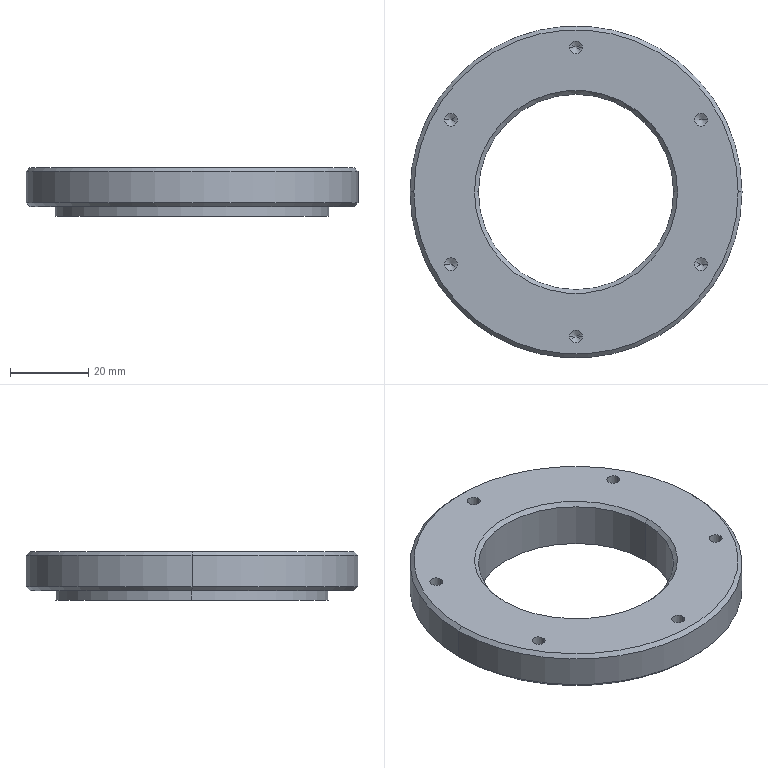Part | SolidWorks | features 3DProfileFeature 1, Chamfer 1, Extrusion 1, HoleWzd 1, ICE 1 | 1 solid | 39 faces | box 85 x 85 x 12.5 mm | volume 41153 mm3 | cylinder 18 | cone 18 | plane 3 | commonest cylinder face diameters 3.3 x12 50 x2 70 x2 85 x2
STEP:
#1=CARTESIAN_POINT('',(-35.,0.,-2.5));
#2=VERTEX_POINT('',#1);
#3=CARTESIAN_POINT('',(35.,0.,-2.5));
#4=VERTEX_POINT('',#3);
#5=CARTESIAN_POINT('',(0.,0.,-2.5));
#6=DIRECTION('',(0.,0.,-1.));
#7=DIRECTION('',(-1.,0.,0.));
#8=AXIS2_PLACEMENT_3D('',#5,#6,#7);
#9=CIRCLE('',#8,35.);
#10=EDGE_CURVE('',#2,#4,#9,.T.);
#11=ORIENTED_EDGE('',*,*,#10,.F.);
#12=CARTESIAN_POINT('',(-35.,0.,0.));
#13=VERTEX_POINT('',#12);
#14=CARTESIAN_POINT('',(-35.,0.,-2.5));
#15=DIRECTION('',(0.,0.,1.));
#16=VECTOR('',#15,1000.);
#17=LINE('',#14,#16);
#18=EDGE_CURVE('',#2,#13,#17,.T.);
#19=ORIENTED_EDGE('',*,*,#18,.T.);
#20=CARTESIAN_POINT('',(35.,0.,0.));
#21=VERTEX_POINT('',#20);
#22=CARTESIAN_POINT('',(0.,0.,0.));
#23=DIRECTION('',(0.,0.,-1.));
#24=DIRECTION('',(1.,0.,0.));
#25=AXIS2_PLACEMENT_3D('',#22,#23,#24);
#26=CIRCLE('',#25,35.);
#27=EDGE_CURVE('',#13,#21,#26,.T.);
#28=ORIENTED_EDGE('',*,*,#27,.T.);
#29=CARTESIAN_POINT('',(35.,0.,-2.5));
#30=DIRECTION('',(0.,0.,1.));
#31=VECTOR('',#30,1000.);
#32=LINE('',#29,#31);
#33=EDGE_CURVE('',#4,#21,#32,.T.);
#34=ORIENTED_EDGE('',*,*,#33,.F.);
#35=EDGE_LOOP('',(#11,#19,#28,#34));
#36=FACE_OUTER_BOUND('',#35,.T.);
#37=CARTESIAN_POINT('',(0.,0.,-2.5));
#38=DIRECTION('',(0.,0.,1.));
#39=DIRECTION('',(1.,0.,0.));
#40=AXIS2_PLACEMENT_3D('',#37,#38,#39);
#41=CYLINDRICAL_SURFACE('',#40,35.);
#42=ADVANCED_FACE('',(#36),#41,.T.);
#43=CARTESIAN_POINT('',(-1.65,37.,4.));
#44=VERTEX_POINT('',#43);
#45=CARTESIAN_POINT('',(1.65,37.,4.));
#46=VERTEX_POINT('',#45);
#47=CARTESIAN_POINT('',(0.,37.,4.));
#48=DIRECTION('',(0.,0.,1.));
#49=DIRECTION('',(1.,0.,0.));
#50=AXIS2_PLACEMENT_3D('',#47,#48,#49);
#51=CIRCLE('',#50,1.65);
#52=EDGE_CURVE('',#44,#46,#51,.T.);
#53=ORIENTED_EDGE('',*,*,#52,.F.);
#54=CARTESIAN_POINT('',(-1.65,37.,10.));
#55=VERTEX_POINT('',#54);
#56=CARTESIAN_POINT('',(-1.65,37.,10.));
#57=DIRECTION('',(0.,0.,1.));
#58=VECTOR('',#57,1000.);
#59=LINE('',#56,#58);
#60=EDGE_CURVE('',#44,#55,#59,.T.);
#61=ORIENTED_EDGE('',*,*,#60,.T.);
#62=CARTESIAN_POINT('',(1.65,37.,10.));
#63=VERTEX_POINT('',#62);
#64=CARTESIAN_POINT('',(0.,37.,10.));
#65=DIRECTION('',(0.,0.,1.));
#66=DIRECTION('',(1.,0.,0.));
#67=AXIS2_PLACEMENT_3D('',#64,#65,#66);
#68=CIRCLE('',#67,1.65);
#69=EDGE_CURVE('',#55,#63,#68,.T.);
#70=ORIENTED_EDGE('',*,*,#69,.T.);
#71=CARTESIAN_POINT('',(1.65,37.,10.));
#72=DIRECTION('',(0.,0.,1.));
#73=VECTOR('',#72,1000.);
#74=LINE('',#71,#73);
#75=EDGE_CURVE('',#46,#63,#74,.T.);
#76=ORIENTED_EDGE('',*,*,#75,.F.);
#77=EDGE_LOOP('',(#53,#61,#70,#76));
#78=FACE_OUTER_BOUND('',#77,.T.);
#79=CARTESIAN_POINT('',(0.,37.,10.));
#80=DIRECTION('',(0.,0.,1.));
#81=DIRECTION('',(1.,0.,0.));
#82=AXIS2_PLACEMENT_3D('',#79,#80,#81);
#83=CYLINDRICAL_SURFACE('',#82,1.65);
#84=ADVANCED_FACE('',(#78),#83,.F.);
#85=CARTESIAN_POINT('',(0.,37.,3.009));
#86=VERTEX_POINT('',#85);
#87=CARTESIAN_POINT('',(1.65,37.,4.));
#88=DIRECTION('',(0.8572,0.,0.515));
#89=VECTOR('',#88,1000.);
#90=LINE('',#87,#89);
#91=EDGE_CURVE('',#86,#46,#90,.T.);
#92=ORIENTED_EDGE('',*,*,#91,.F.);
#93=CARTESIAN_POINT('',(-1.65,37.,4.));
#94=DIRECTION('',(-0.8572,0.,0.515));
#95=VECTOR('',#94,1000.);
#96=LINE('',#93,#95);
#97=EDGE_CURVE('',#86,#44,#96,.T.);
#98=ORIENTED_EDGE('',*,*,#97,.T.);
#99=ORIENTED_EDGE('',*,*,#52,.T.);
#100=EDGE_LOOP('',(#92,#98,#99));
#101=FACE_OUTER_BOUND('',#100,.T.);
#102=CARTESIAN_POINT('',(0.,37.,4.));
#103=DIRECTION('',(0.,0.,1.));
#104=DIRECTION('',(1.,0.,0.));
#105=AXIS2_PLACEMENT_3D('',#102,#103,#104);
#106=CONICAL_SURFACE('',#105,1.65,1.03);
#107=ADVANCED_FACE('',(#101),#106,.F.);
#108=CARTESIAN_POINT('',(30.393,18.501,4.));
#109=VERTEX_POINT('',#108);
#110=CARTESIAN_POINT('',(33.693,18.501,4.));
#111=VERTEX_POINT('',#110);
#112=CARTESIAN_POINT('',(32.043,18.501,4.));
#113=DIRECTION('',(0.,0.,1.));
#114=DIRECTION('',(1.,0.,0.));
#115=AXIS2_PLACEMENT_3D('',#112,#113,#114);
#116=CIRCLE('',#115,1.65);
#117=EDGE_CURVE('',#109,#111,#116,.T.);
#118=ORIENTED_EDGE('',*,*,#117,.F.);
#119=CARTESIAN_POINT('',(30.393,18.501,10.));
#120=VERTEX_POINT('',#119);
#121=CARTESIAN_POINT('',(30.393,18.501,10.));
#122=DIRECTION('',(0.,0.,1.));
#123=VECTOR('',#122,1000.);
#124=LINE('',#121,#123);
#125=EDGE_CURVE('',#109,#120,#124,.T.);
#126=ORIENTED_EDGE('',*,*,#125,.T.);
#127=CARTESIAN_POINT('',(33.693,18.501,10.));
#128=VERTEX_POINT('',#127);
#129=CARTESIAN_POINT('',(32.043,18.501,10.));
#130=DIRECTION('',(0.,0.,1.));
#131=DIRECTION('',(1.,0.,0.));
#132=AXIS2_PLACEMENT_3D('',#129,#130,#131);
#133=CIRCLE('',#132,1.65);
#134=EDGE_CURVE('',#120,#128,#133,.T.);
#135=ORIENTED_EDGE('',*,*,#134,.T.);
#136=CARTESIAN_POINT('',(33.693,18.501,10.));
#137=DIRECTION('',(0.,0.,1.));
#138=VECTOR('',#137,1000.);
#139=LINE('',#136,#138);
#140=EDGE_CURVE('',#111,#128,#139,.T.);
#141=ORIENTED_EDGE('',*,*,#140,.F.);
#142=EDGE_LOOP('',(#118,#126,#135,#141));
#143=FACE_OUTER_BOUND('',#142,.T.);
#144=CARTESIAN_POINT('',(32.043,18.501,10.));
#145=DIRECTION('',(0.,0.,1.));
#146=DIRECTION('',(1.,0.,0.));
#147=AXIS2_PLACEMENT_3D('',#144,#145,#146);
#148=CYLINDRICAL_SURFACE('',#147,1.65);
#149=ADVANCED_FACE('',(#143),#148,.F.);
#150=CARTESIAN_POINT('',(32.043,18.501,3.009));
#151=VERTEX_POINT('',#150);
#152=CARTESIAN_POINT('',(33.693,18.501,4.));
#153=DIRECTION('',(0.8572,0.,0.515));
#154=VECTOR('',#153,1000.);
#155=LINE('',#152,#154);
#156=EDGE_CURVE('',#151,#111,#155,.T.);
#157=ORIENTED_EDGE('',*,*,#156,.F.);
#158=CARTESIAN_POINT('',(30.393,18.501,4.));
#159=DIRECTION('',(-0.8572,0.,0.515));
#160=VECTOR('',#159,1000.);
#161=LINE('',#158,#160);
#162=EDGE_CURVE('',#151,#109,#161,.T.);
#163=ORIENTED_EDGE('',*,*,#162,.T.);
#164=ORIENTED_EDGE('',*,*,#117,.T.);
#165=EDGE_LOOP('',(#157,#163,#164));
#166=FACE_OUTER_BOUND('',#165,.T.);
#167=CARTESIAN_POINT('',(32.043,18.501,4.));
#168=DIRECTION('',(0.,0.,1.));
#169=DIRECTION('',(1.,0.,0.));
#170=AXIS2_PLACEMENT_3D('',#167,#168,#169);
#171=CONICAL_SURFACE('',#170,1.65,1.03);
#172=ADVANCED_FACE('',(#166),#171,.F.);
#173=CARTESIAN_POINT('',(30.394,-18.499,4.));
#174=VERTEX_POINT('',#173);
#175=CARTESIAN_POINT('',(33.694,-18.499,4.));
#176=VERTEX_POINT('',#175);
#177=CARTESIAN_POINT('',(32.044,-18.499,4.));
#178=DIRECTION('',(0.,0.,1.));
#179=DIRECTION('',(1.,0.,0.));
#180=AXIS2_PLACEMENT_3D('',#177,#178,#179);
#181=CIRCLE('',#180,1.65);
#182=EDGE_CURVE('',#174,#176,#181,.T.);
#183=ORIENTED_EDGE('',*,*,#182,.F.);
#184=CARTESIAN_POINT('',(30.394,-18.499,10.));
#185=VERTEX_POINT('',#184);
#186=CARTESIAN_POINT('',(30.394,-18.499,10.));
#187=DIRECTION('',(0.,0.,1.));
#188=VECTOR('',#187,1000.);
#189=LINE('',#186,#188);
#190=EDGE_CURVE('',#174,#185,#189,.T.);
#191=ORIENTED_EDGE('',*,*,#190,.T.);
#192=CARTESIAN_POINT('',(33.694,-18.499,10.));
#193=VERTEX_POINT('',#192);
#194=CARTESIAN_POINT('',(32.044,-18.499,10.));
#195=DIRECTION('',(0.,0.,1.));
#196=DIRECTION('',(1.,0.,0.));
#197=AXIS2_PLACEMENT_3D('',#194,#195,#196);
#198=CIRCLE('',#197,1.65);
#199=EDGE_CURVE('',#185,#193,#198,.T.);
#200=ORIENTED_EDGE('',*,*,#199,.T.);
#201=CARTESIAN_POINT('',(33.694,-18.499,10.));
#202=DIRECTION('',(0.,0.,1.));
#203=VECTOR('',#202,1000.);
#204=LINE('',#201,#203);
#205=EDGE_CURVE('',#176,#193,#204,.T.);
#206=ORIENTED_EDGE('',*,*,#205,.F.);
#207=EDGE_LOOP('',(#183,#191,#200,#206));
#208=FACE_OUTER_BOUND('',#207,.T.);
#209=CARTESIAN_POINT('',(32.044,-18.499,10.));
#210=DIRECTION('',(0.,0.,1.));
#211=DIRECTION('',(1.,0.,0.));
#212=AXIS2_PLACEMENT_3D('',#209,#210,#211);
#213=CYLINDRICAL_SURFACE('',#212,1.65);
#214=ADVANCED_FACE('',(#208),#213,.F.);
#215=CARTESIAN_POINT('',(32.044,-18.499,3.009));
#216=VERTEX_POINT('',#215);
#217=CARTESIAN_POINT('',(33.694,-18.499,4.));
#218=DIRECTION('',(0.8572,0.,0.515));
#219=VECTOR('',#218,1000.);
#220=LINE('',#217,#219);
#221=EDGE_CURVE('',#216,#176,#220,.T.);
#222=ORIENTED_EDGE('',*,*,#221,.F.);
#223=CARTESIAN_POINT('',(30.394,-18.499,4.));
#224=DIRECTION('',(-0.8572,0.,0.515));
#225=VECTOR('',#224,1000.);
#226=LINE('',#223,#225);
#227=EDGE_CURVE('',#216,#174,#226,.T.);
#228=ORIENTED_EDGE('',*,*,#227,.T.);
#229=ORIENTED_EDGE('',*,*,#182,.T.);
#230=EDGE_LOOP('',(#222,#228,#229));
#231=FACE_OUTER_BOUND('',#230,.T.);
#232=CARTESIAN_POINT('',(32.044,-18.499,4.));
#233=DIRECTION('',(0.,0.,1.));
#234=DIRECTION('',(1.,0.,0.));
#235=AXIS2_PLACEMENT_3D('',#232,#233,#234);
#236=CONICAL_SURFACE('',#235,1.65,1.03);
#237=ADVANCED_FACE('',(#231),#236,.F.);
#238=CARTESIAN_POINT('',(-1.648,-37.,4.));
#239=VERTEX_POINT('',#238);
#240=CARTESIAN_POINT('',(1.652,-37.,4.));
#241=VERTEX_POINT('',#240);
#242=CARTESIAN_POINT('',(0.002,-37.,4.));
#243=DIRECTION('',(0.,0.,1.));
#244=DIRECTION('',(1.,0.,0.));
#245=AXIS2_PLACEMENT_3D('',#242,#243,#244);
#246=CIRCLE('',#245,1.65);
#247=EDGE_CURVE('',#239,#241,#246,.T.);
#248=ORIENTED_EDGE('',*,*,#247,.F.);
#249=CARTESIAN_POINT('',(-1.648,-37.,10.));
#250=VERTEX_POINT('',#249);
#251=CARTESIAN_POINT('',(-1.648,-37.,10.));
#252=DIRECTION('',(0.,0.,1.));
#253=VECTOR('',#252,1000.);
#254=LINE('',#251,#253);
#255=EDGE_CURVE('',#239,#250,#254,.T.);
#256=ORIENTED_EDGE('',*,*,#255,.T.);
#257=CARTESIAN_POINT('',(1.652,-37.,10.));
#258=VERTEX_POINT('',#257);
#259=CARTESIAN_POINT('',(0.002,-37.,10.));
#260=DIRECTION('',(0.,0.,1.));
#261=DIRECTION('',(1.,0.,0.));
#262=AXIS2_PLACEMENT_3D('',#259,#260,#261);
#263=CIRCLE('',#262,1.65);
#264=EDGE_CURVE('',#250,#258,#263,.T.);
#265=ORIENTED_EDGE('',*,*,#264,.T.);
#266=CARTESIAN_POINT('',(1.652,-37.,10.));
#267=DIRECTION('',(0.,0.,1.));
#268=VECTOR('',#267,1000.);
#269=LINE('',#266,#268);
#270=EDGE_CURVE('',#241,#258,#269,.T.);
#271=ORIENTED_EDGE('',*,*,#270,.F.);
#272=EDGE_LOOP('',(#248,#256,#265,#271));
#273=FACE_OUTER_BOUND('',#272,.T.);
#274=CARTESIAN_POINT('',(0.002,-37.,10.));
#275=DIRECTION('',(0.,0.,1.));
#276=DIRECTION('',(1.,0.,0.));
#277=AXIS2_PLACEMENT_3D('',#274,#275,#276);
#278=CYLINDRICAL_SURFACE('',#277,1.65);
#279=ADVANCED_FACE('',(#273),#278,.F.);
#280=CARTESIAN_POINT('',(0.002,-37.,3.009));
#281=VERTEX_POINT('',#280);
#282=CARTESIAN_POINT('',(1.652,-37.,4.));
#283=DIRECTION('',(0.8572,0.,0.515));
#284=VECTOR('',#283,1000.);
#285=LINE('',#282,#284);
#286=EDGE_CURVE('',#281,#241,#285,.T.);
#287=ORIENTED_EDGE('',*,*,#286,.F.);
#288=CARTESIAN_POINT('',(-1.648,-37.,4.));
#289=DIRECTION('',(-0.8572,0.,0.515));
#290=VECTOR('',#289,1000.);
#291=LINE('',#288,#290);
#292=EDGE_CURVE('',#281,#239,#291,.T.);
#293=ORIENTED_EDGE('',*,*,#292,.T.);
#294=ORIENTED_EDGE('',*,*,#247,.T.);
#295=EDGE_LOOP('',(#287,#293,#294));
#296=FACE_OUTER_BOUND('',#295,.T.);
#297=CARTESIAN_POINT('',(0.002,-37.,4.));
#298=DIRECTION('',(0.,0.,1.));
#299=DIRECTION('',(1.,0.,0.));
#300=AXIS2_PLACEMENT_3D('',#297,#298,#299);
#301=CONICAL_SURFACE('',#300,1.65,1.03);
#302=ADVANCED_FACE('',(#296),#301,.F.);
#303=CARTESIAN_POINT('',(-33.691,-18.501,4.));
#304=VERTEX_POINT('',#303);
#305=CARTESIAN_POINT('',(-30.391,-18.501,4.));
#306=VERTEX_POINT('',#305);
#307=CARTESIAN_POINT('',(-32.041,-18.501,4.));
#308=DIRECTION('',(0.,0.,1.));
#309=DIRECTION('',(1.,0.,0.));
#310=AXIS2_PLACEMENT_3D('',#307,#308,#309);
#311=CIRCLE('',#310,1.65);
#312=EDGE_CURVE('',#304,#306,#311,.T.);
#313=ORIENTED_EDGE('',*,*,#312,.F.);
#314=CARTESIAN_POINT('',(-33.691,-18.501,10.));
#315=VERTEX_POINT('',#314);
#316=CARTESIAN_POINT('',(-33.691,-18.501,10.));
#317=DIRECTION('',(0.,0.,1.));
#318=VECTOR('',#317,1000.);
#319=LINE('',#316,#318);
#320=EDGE_CURVE('',#304,#315,#319,.T.);
#321=ORIENTED_EDGE('',*,*,#320,.T.);
#322=CARTESIAN_POINT('',(-30.391,-18.501,10.));
#323=VERTEX_POINT('',#322);
#324=CARTESIAN_POINT('',(-32.041,-18.501,10.));
#325=DIRECTION('',(0.,0.,1.));
#326=DIRECTION('',(1.,0.,0.));
#327=AXIS2_PLACEMENT_3D('',#324,#325,#326);
#328=CIRCLE('',#327,1.65);
#329=EDGE_CURVE('',#315,#323,#328,.T.);
#330=ORIENTED_EDGE('',*,*,#329,.T.);
#331=CARTESIAN_POINT('',(-30.391,-18.501,10.));
#332=DIRECTION('',(0.,0.,1.));
#333=VECTOR('',#332,1000.);
#334=LINE('',#331,#333);
#335=EDGE_CURVE('',#306,#323,#334,.T.);
#336=ORIENTED_EDGE('',*,*,#335,.F.);
#337=EDGE_LOOP('',(#313,#321,#330,#336));
#338=FACE_OUTER_BOUND('',#337,.T.);
#339=CARTESIAN_POINT('',(-32.041,-18.501,10.));
#340=DIRECTION('',(0.,0.,1.));
#341=DIRECTION('',(1.,0.,0.));
#342=AXIS2_PLACEMENT_3D('',#339,#340,#341);
#343=CYLINDRICAL_SURFACE('',#342,1.65);
#344=ADVANCED_FACE('',(#338),#343,.F.);
#345=CARTESIAN_POINT('',(-32.041,-18.501,3.009));
#346=VERTEX_POINT('',#345);
#347=CARTESIAN_POINT('',(-30.391,-18.501,4.));
#348=DIRECTION('',(0.8572,0.,0.515));
#349=VECTOR('',#348,1000.);
#350=LINE('',#347,#349);
#351=EDGE_CURVE('',#346,#306,#350,.T.);
#352=ORIENTED_EDGE('',*,*,#351,.F.);
#353=CARTESIAN_POINT('',(-33.691,-18.501,4.));
#354=DIRECTION('',(-0.8572,0.,0.515));
#355=VECTOR('',#354,1000.);
#356=LINE('',#353,#355);
#357=EDGE_CURVE('',#346,#304,#356,.T.);
#358=ORIENTED_EDGE('',*,*,#357,.T.);
#359=ORIENTED_EDGE('',*,*,#312,.T.);
#360=EDGE_LOOP('',(#352,#358,#359));
#361=FACE_OUTER_BOUND('',#360,.T.);
#362=CARTESIAN_POINT('',(-32.041,-18.501,4.));
#363=DIRECTION('',(0.,0.,1.));
#364=DIRECTION('',(1.,0.,0.));
#365=AXIS2_PLACEMENT_3D('',#362,#363,#364);
#366=CONICAL_SURFACE('',#365,1.65,1.03);
#367=ADVANCED_FACE('',(#361),#366,.F.);
#368=CARTESIAN_POINT('',(-33.692,18.499,4.));
#369=VERTEX_POINT('',#368);
#370=CARTESIAN_POINT('',(-30.392,18.499,4.));
#371=VERTEX_POINT('',#370);
#372=CARTESIAN_POINT('',(-32.042,18.499,4.));
#373=DIRECTION('',(0.,0.,1.));
#374=DIRECTION('',(1.,0.,0.));
#375=AXIS2_PLACEMENT_3D('',#372,#373,#374);
#376=CIRCLE('',#375,1.65);
#377=EDGE_CURVE('',#369,#371,#376,.T.);
#378=ORIENTED_EDGE('',*,*,#377,.F.);
#379=CARTESIAN_POINT('',(-33.692,18.499,10.));
#380=VERTEX_POINT('',#379);
#381=CARTESIAN_POINT('',(-33.692,18.499,10.));
#382=DIRECTION('',(0.,0.,1.));
#383=VECTOR('',#382,1000.);
#384=LINE('',#381,#383);
#385=EDGE_CURVE('',#369,#380,#384,.T.);
#386=ORIENTED_EDGE('',*,*,#385,.T.);
#387=CARTESIAN_POINT('',(-30.392,18.499,10.));
#388=VERTEX_POINT('',#387);
#389=CARTESIAN_POINT('',(-32.042,18.499,10.));
#390=DIRECTION('',(0.,0.,1.));
#391=DIRECTION('',(1.,0.,0.));
#392=AXIS2_PLACEMENT_3D('',#389,#390,#391);
#393=CIRCLE('',#392,1.65);
#394=EDGE_CURVE('',#380,#388,#393,.T.);
#395=ORIENTED_EDGE('',*,*,#394,.T.);
#396=CARTESIAN_POINT('',(-30.392,18.499,10.));
#397=DIRECTION('',(0.,0.,1.));
#398=VECTOR('',#397,1000.);
#399=LINE('',#396,#398);
#400=EDGE_CURVE('',#371,#388,#399,.T.);
#401=ORIENTED_EDGE('',*,*,#400,.F.);
#402=EDGE_LOOP('',(#378,#386,#395,#401));
#403=FACE_OUTER_BOUND('',#402,.T.);
#404=CARTESIAN_POINT('',(-32.042,18.499,10.));
#405=DIRECTION('',(0.,0.,1.));
#406=DIRECTION('',(1.,0.,0.));
#407=AXIS2_PLACEMENT_3D('',#404,#405,#406);
#408=CYLINDRICAL_SURFACE('',#407,1.65);
#409=ADVANCED_FACE('',(#403),#408,.F.);
#410=CARTESIAN_POINT('',(-32.042,18.499,3.009));
#411=VERTEX_POINT('',#410);
#412=CARTESIAN_POINT('',(-30.392,18.499,4.));
#413=DIRECTION('',(0.8572,0.,0.515));
#414=VECTOR('',#413,1000.);
#415=LINE('',#412,#414);
#416=EDGE_CURVE('',#411,#371,#415,.T.);
#417=ORIENTED_EDGE('',*,*,#416,.F.);
#418=CARTESIAN_POINT('',(-33.692,18.499,4.));
#419=DIRECTION('',(-0.8572,0.,0.515));
#420=VECTOR('',#419,1000.);
#421=LINE('',#418,#420);
#422=EDGE_CURVE('',#411,#369,#421,.T.);
#423=ORIENTED_EDGE('',*,*,#422,.T.);
#424=ORIENTED_EDGE('',*,*,#377,.T.);
#425=EDGE_LOOP('',(#417,#423,#424));
#426=FACE_OUTER_BOUND('',#425,.T.);
#427=CARTESIAN_POINT('',(-32.042,18.499,4.));
#428=DIRECTION('',(0.,0.,1.));
#429=DIRECTION('',(1.,0.,0.));
#430=AXIS2_PLACEMENT_3D('',#427,#428,#429);
#431=CONICAL_SURFACE('',#430,1.65,1.03);
#432=ADVANCED_FACE('',(#426),#431,.F.);
#433=CARTESIAN_POINT('',(41.5,0.,10.));
#434=VERTEX_POINT('',#433);
#435=CARTESIAN_POINT('',(-41.5,0.,10.));
#436=VERTEX_POINT('',#435);
#437=CARTESIAN_POINT('',(0.,0.,10.));
#438=DIRECTION('',(0.,0.,1.));
#439=DIRECTION('',(1.,0.,0.));
#440=AXIS2_PLACEMENT_3D('',#437,#438,#439);
#441=CIRCLE('',#440,41.5);
#442=EDGE_CURVE('',#434,#436,#441,.T.);
#443=ORIENTED_EDGE('',*,*,#442,.F.);
#444=CARTESIAN_POINT('',(42.5,0.,9.));
#445=VERTEX_POINT('',#444);
#446=CARTESIAN_POINT('',(41.5,0.,10.));
#447=DIRECTION('',(0.7071,0.,-0.7071));
#448=VECTOR('',#447,1000.);
#449=LINE('',#446,#448);
#450=EDGE_CURVE('',#434,#445,#449,.T.);
#451=ORIENTED_EDGE('',*,*,#450,.T.);
#452=CARTESIAN_POINT('',(-42.5,0.,9.));
#453=VERTEX_POINT('',#452);
#454=CARTESIAN_POINT('',(0.,0.,9.));
#455=DIRECTION('',(0.,0.,-1.));
#456=DIRECTION('',(1.,0.,0.));
#457=AXIS2_PLACEMENT_3D('',#454,#455,#456);
#458=CIRCLE('',#457,42.5);
#459=EDGE_CURVE('',#453,#445,#458,.T.);
#460=ORIENTED_EDGE('',*,*,#459,.F.);
#461=CARTESIAN_POINT('',(-41.5,0.,10.));
#462=DIRECTION('',(-0.7071,0.,-0.7071));
#463=VECTOR('',#462,1000.);
#464=LINE('',#461,#463);
#465=EDGE_CURVE('',#436,#453,#464,.T.);
#466=ORIENTED_EDGE('',*,*,#465,.F.);
#467=EDGE_LOOP('',(#443,#451,#460,#466));
#468=FACE_OUTER_BOUND('',#467,.T.);
#469=CARTESIAN_POINT('',(0.,0.,10.));
#470=DIRECTION('',(0.,0.,-1.));
#471=DIRECTION('',(-1.,0.,0.));
#472=AXIS2_PLACEMENT_3D('',#469,#470,#471);
#473=CONICAL_SURFACE('',#472,41.5,0.7854);
#474=ADVANCED_FACE('',(#468),#473,.T.);
#475=CARTESIAN_POINT('',(-41.5,0.,0.));
#476=VERTEX_POINT('',#475);
#477=CARTESIAN_POINT('',(41.5,0.,0.));
#478=VERTEX_POINT('',#477);
#479=CARTESIAN_POINT('',(0.,0.,0.));
#480=DIRECTION('',(0.,0.,-1.));
#481=DIRECTION('',(1.,0.,0.));
#482=AXIS2_PLACEMENT_3D('',#479,#480,#481);
#483=CIRCLE('',#482,41.5);
#484=EDGE_CURVE('',#476,#478,#483,.T.);
#485=ORIENTED_EDGE('',*,*,#484,.F.);
#486=CARTESIAN_POINT('',(-42.5,0.,1.));
#487=VERTEX_POINT('',#486);
#488=CARTESIAN_POINT('',(-42.5,0.,1.));
#489=DIRECTION('',(-0.7071,0.,0.7071));
#490=VECTOR('',#489,1000.);
#491=LINE('',#488,#490);
#492=EDGE_CURVE('',#476,#487,#491,.T.);
#493=ORIENTED_EDGE('',*,*,#492,.T.);
#494=CARTESIAN_POINT('',(42.5,0.,1.));
#495=VERTEX_POINT('',#494);
#496=CARTESIAN_POINT('',(0.,0.,1.));
#497=DIRECTION('',(0.,0.,1.));
#498=DIRECTION('',(1.,0.,0.));
#499=AXIS2_PLACEMENT_3D('',#496,#497,#498);
#500=CIRCLE('',#499,42.5);
#501=EDGE_CURVE('',#495,#487,#500,.T.);
#502=ORIENTED_EDGE('',*,*,#501,.F.);
#503=CARTESIAN_POINT('',(42.5,0.,1.));
#504=DIRECTION('',(0.7071,0.,0.7071));
#505=VECTOR('',#504,1000.);
#506=LINE('',#503,#505);
#507=EDGE_CURVE('',#478,#495,#506,.T.);
#508=ORIENTED_EDGE('',*,*,#507,.F.);
#509=EDGE_LOOP('',(#485,#493,#502,#508));
#510=FACE_OUTER_BOUND('',#509,.T.);
#511=CARTESIAN_POINT('',(0.,0.,1.));
#512=DIRECTION('',(0.,0.,1.));
#513=DIRECTION('',(1.,0.,0.));
#514=AXIS2_PLACEMENT_3D('',#511,#512,#513);
#515=CONICAL_SURFACE('',#514,42.5,0.7854);
#516=ADVANCED_FACE('',(#510),#515,.T.);
#517=CARTESIAN_POINT('',(-25.,0.,9.));
#518=VERTEX_POINT('',#517);
#519=CARTESIAN_POINT('',(25.,0.,9.));
#520=VERTEX_POINT('',#519);
#521=CARTESIAN_POINT('',(0.,0.,9.));
#522=DIRECTION('',(0.,0.,1.));
#523=DIRECTION('',(1.,0.,0.));
#524=AXIS2_PLACEMENT_3D('',#521,#522,#523);
#525=CIRCLE('',#524,25.);
#526=EDGE_CURVE('',#518,#520,#525,.T.);
#527=ORIENTED_EDGE('',*,*,#526,.F.);
#528=CARTESIAN_POINT('',(-26.,0.,10.));
#529=VERTEX_POINT('',#528);
#530=CARTESIAN_POINT('',(-25.,0.,9.));
#531=DIRECTION('',(-0.7071,0.,0.7071));
#532=VECTOR('',#531,1000.);
#533=LINE('',#530,#532);
#534=EDGE_CURVE('',#518,#529,#533,.T.);
#535=ORIENTED_EDGE('',*,*,#534,.T.);
#536=CARTESIAN_POINT('',(26.,0.,10.));
#537=VERTEX_POINT('',#536);
#538=CARTESIAN_POINT('',(0.,0.,10.));
#539=DIRECTION('',(0.,0.,-1.));
#540=DIRECTION('',(1.,0.,0.));
#541=AXIS2_PLACEMENT_3D('',#538,#539,#540);
#542=CIRCLE('',#541,26.);
#543=EDGE_CURVE('',#537,#529,#542,.T.);
#544=ORIENTED_EDGE('',*,*,#543,.F.);
#545=CARTESIAN_POINT('',(25.,0.,9.));
#546=DIRECTION('',(0.7071,0.,0.7071));
#547=VECTOR('',#546,1000.);
#548=LINE('',#545,#547);
#549=EDGE_CURVE('',#520,#537,#548,.T.);
#550=ORIENTED_EDGE('',*,*,#549,.F.);
#551=EDGE_LOOP('',(#527,#535,#544,#550));
#552=FACE_OUTER_BOUND('',#551,.T.);
#553=CARTESIAN_POINT('',(0.,0.,9.));
#554=DIRECTION('',(0.,0.,1.));
#555=DIRECTION('',(1.,0.,0.));
#556=AXIS2_PLACEMENT_3D('',#553,#554,#555);
#557=CONICAL_SURFACE('',#556,25.,0.7854);
#558=ADVANCED_FACE('',(#552),#557,.F.);
#559=ORIENTED_EDGE('',*,*,#526,.T.);
#560=CARTESIAN_POINT('',(25.,0.,-2.5));
#561=VERTEX_POINT('',#560);
#562=CARTESIAN_POINT('',(25.,0.,10.));
#563=DIRECTION('',(0.,0.,-1.));
#564=VECTOR('',#563,1000.);
#565=LINE('',#562,#564);
#566=EDGE_CURVE('',#520,#561,#565,.T.);
#567=ORIENTED_EDGE('',*,*,#566,.T.);
#568=CARTESIAN_POINT('',(-25.,0.,-2.5));
#569=VERTEX_POINT('',#568);
#570=CARTESIAN_POINT('',(0.,0.,-2.5));
#571=DIRECTION('',(0.,0.,-1.));
#572=DIRECTION('',(-1.,0.,0.));
#573=AXIS2_PLACEMENT_3D('',#570,#571,#572);
#574=CIRCLE('',#573,25.);
#575=EDGE_CURVE('',#561,#569,#574,.T.);
#576=ORIENTED_EDGE('',*,*,#575,.T.);
#577=CARTESIAN_POINT('',(-25.,0.,10.));
#578=DIRECTION('',(0.,0.,-1.));
#579=VECTOR('',#578,1000.);
#580=LINE('',#577,#579);
#581=EDGE_CURVE('',#518,#569,#580,.T.);
#582=ORIENTED_EDGE('',*,*,#581,.F.);
#583=EDGE_LOOP('',(#559,#567,#576,#582));
#584=FACE_OUTER_BOUND('',#583,.T.);
#585=CARTESIAN_POINT('',(0.,0.,10.));
#586=DIRECTION('',(0.,0.,-1.));
#587=DIRECTION('',(-1.,0.,0.));
#588=AXIS2_PLACEMENT_3D('',#585,#586,#587);
#589=CYLINDRICAL_SURFACE('',#588,25.);
#590=ADVANCED_FACE('',(#584),#589,.F.);
#591=ORIENTED_EDGE('',*,*,#459,.T.);
#592=CARTESIAN_POINT('',(42.5,0.,10.));
#593=DIRECTION('',(0.,0.,-1.));
#594=VECTOR('',#593,1000.);
#595=LINE('',#592,#594);
#596=EDGE_CURVE('',#445,#495,#595,.T.);
#597=ORIENTED_EDGE('',*,*,#596,.T.);
#598=ORIENTED_EDGE('',*,*,#501,.T.);
#599=CARTESIAN_POINT('',(-42.5,0.,10.));
#600=DIRECTION('',(0.,0.,-1.));
#601=VECTOR('',#600,1000.);
#602=LINE('',#599,#601);
#603=EDGE_CURVE('',#453,#487,#602,.T.);
#604=ORIENTED_EDGE('',*,*,#603,.F.);
#605=EDGE_LOOP('',(#591,#597,#598,#604));
#606=FACE_OUTER_BOUND('',#605,.T.);
#607=CARTESIAN_POINT('',(0.,0.,10.));
#608=DIRECTION('',(0.,0.,-1.));
#609=DIRECTION('',(-1.,0.,0.));
#610=AXIS2_PLACEMENT_3D('',#607,#608,#609);
#611=CYLINDRICAL_SURFACE('',#610,42.5);
#612=ADVANCED_FACE('',(#606),#611,.T.);
#613=CARTESIAN_POINT('',(0.,0.,0.));
#614=DIRECTION('',(0.,0.,-1.));
#615=DIRECTION('',(1.,0.,0.));
#616=AXIS2_PLACEMENT_3D('',#613,#614,#615);
#617=CIRCLE('',#616,41.5);
#618=EDGE_CURVE('',#478,#476,#617,.T.);
#619=ORIENTED_EDGE('',*,*,#618,.T.);
#620=ORIENTED_EDGE('',*,*,#484,.T.);
#621=EDGE_LOOP('',(#619,#620));
#622=FACE_OUTER_BOUND('',#621,.T.);
#623=CARTESIAN_POINT('',(0.,0.,0.));
#624=DIRECTION('',(0.,0.,-1.));
#625=DIRECTION('',(1.,0.,0.));
#626=AXIS2_PLACEMENT_3D('',#623,#624,#625);
#627=CIRCLE('',#626,35.);
#628=EDGE_CURVE('',#21,#13,#627,.T.);
#629=ORIENTED_EDGE('',*,*,#628,.F.);
#630=ORIENTED_EDGE('',*,*,#27,.F.);
#631=EDGE_LOOP('',(#629,#630));
#632=FACE_BOUND('',#631,.T.);
#633=CARTESIAN_POINT('',(0.,0.,0.));
#634=DIRECTION('',(0.,0.,1.));
#635=DIRECTION('',(1.,0.,0.));
#636=AXIS2_PLACEMENT_3D('',#633,#634,#635);
#637=PLANE('',#636);
#638=ADVANCED_FACE('',(#622,#632),#637,.F.);
#639=CARTESIAN_POINT('',(0.,37.,10.));
#640=DIRECTION('',(0.,0.,1.));
#641=DIRECTION('',(1.,0.,0.));
#642=AXIS2_PLACEMENT_3D('',#639,#640,#641);
#643=CIRCLE('',#642,1.65);
#644=EDGE_CURVE('',#63,#55,#643,.T.);
#645=ORIENTED_EDGE('',*,*,#644,.F.);
#646=ORIENTED_EDGE('',*,*,#69,.F.);
#647=EDGE_LOOP('',(#645,#646));
#648=FACE_BOUND('',#647,.T.);
#649=CARTESIAN_POINT('',(32.043,18.501,10.));
#650=DIRECTION('',(0.,0.,1.));
#651=DIRECTION('',(1.,0.,0.));
#652=AXIS2_PLACEMENT_3D('',#649,#650,#651);
#653=CIRCLE('',#652,1.65);
#654=EDGE_CURVE('',#128,#120,#653,.T.);
#655=ORIENTED_EDGE('',*,*,#654,.F.);
#656=ORIENTED_EDGE('',*,*,#134,.F.);
#657=EDGE_LOOP('',(#655,#656));
#658=FACE_BOUND('',#657,.T.);
#659=CARTESIAN_POINT('',(32.044,-18.499,10.));
#660=DIRECTION('',(0.,0.,1.));
#661=DIRECTION('',(1.,0.,0.));
#662=AXIS2_PLACEMENT_3D('',#659,#660,#661);
#663=CIRCLE('',#662,1.65);
#664=EDGE_CURVE('',#193,#185,#663,.T.);
#665=ORIENTED_EDGE('',*,*,#664,.F.);
#666=ORIENTED_EDGE('',*,*,#199,.F.);
#667=EDGE_LOOP('',(#665,#666));
#668=FACE_BOUND('',#667,.T.);
#669=CARTESIAN_POINT('',(0.002,-37.,10.));
#670=DIRECTION('',(0.,0.,1.));
#671=DIRECTION('',(1.,0.,0.));
#672=AXIS2_PLACEMENT_3D('',#669,#670,#671);
#673=CIRCLE('',#672,1.65);
#674=EDGE_CURVE('',#258,#250,#673,.T.);
#675=ORIENTED_EDGE('',*,*,#674,.F.);
#676=ORIENTED_EDGE('',*,*,#264,.F.);
#677=EDGE_LOOP('',(#675,#676));
#678=FACE_BOUND('',#677,.T.);
#679=CARTESIAN_POINT('',(-32.041,-18.501,10.));
#680=DIRECTION('',(0.,0.,1.));
#681=DIRECTION('',(1.,0.,0.));
#682=AXIS2_PLACEMENT_3D('',#679,#680,#681);
#683=CIRCLE('',#682,1.65);
#684=EDGE_CURVE('',#323,#315,#683,.T.);
#685=ORIENTED_EDGE('',*,*,#684,.F.);
#686=ORIENTED_EDGE('',*,*,#329,.F.);
#687=EDGE_LOOP('',(#685,#686));
#688=FACE_BOUND('',#687,.T.);
#689=CARTESIAN_POINT('',(-32.042,18.499,10.));
#690=DIRECTION('',(0.,0.,1.));
#691=DIRECTION('',(1.,0.,0.));
#692=AXIS2_PLACEMENT_3D('',#689,#690,#691);
#693=CIRCLE('',#692,1.65);
#694=EDGE_CURVE('',#388,#380,#693,.T.);
#695=ORIENTED_EDGE('',*,*,#694,.F.);
#696=ORIENTED_EDGE('',*,*,#394,.F.);
#697=EDGE_LOOP('',(#695,#696));
#698=FACE_BOUND('',#697,.T.);
#699=ORIENTED_EDGE('',*,*,#543,.T.);
#700=CARTESIAN_POINT('',(0.,0.,10.));
#701=DIRECTION('',(0.,0.,-1.));
#702=DIRECTION('',(1.,0.,0.));
#703=AXIS2_PLACEMENT_3D('',#700,#701,#702);
#704=CIRCLE('',#703,26.);
#705=EDGE_CURVE('',#529,#537,#704,.T.);
#706=ORIENTED_EDGE('',*,*,#705,.T.);
#707=EDGE_LOOP('',(#699,#706));
#708=FACE_BOUND('',#707,.T.);
#709=CARTESIAN_POINT('',(0.,0.,10.));
#710=DIRECTION('',(0.,0.,1.));
#711=DIRECTION('',(1.,0.,0.));
#712=AXIS2_PLACEMENT_3D('',#709,#710,#711);
#713=CIRCLE('',#712,41.5);
#714=EDGE_CURVE('',#436,#434,#713,.T.);
#715=ORIENTED_EDGE('',*,*,#714,.T.);
#716=ORIENTED_EDGE('',*,*,#442,.T.);
#717=EDGE_LOOP('',(#715,#716));
#718=FACE_OUTER_BOUND('',#717,.T.);
#719=CARTESIAN_POINT('',(0.,0.,10.));
#720=DIRECTION('',(0.,0.,1.));
#721=DIRECTION('',(1.,0.,0.));
#722=AXIS2_PLACEMENT_3D('',#719,#720,#721);
#723=PLANE('',#722);
#724=ADVANCED_FACE('',(#648,#658,#668,#678,#688,#698,#708,#718),#723,.T.);
#725=ORIENTED_EDGE('',*,*,#596,.F.);
#726=CARTESIAN_POINT('',(0.,0.,9.));
#727=DIRECTION('',(0.,0.,-1.));
#728=DIRECTION('',(1.,0.,0.));
#729=AXIS2_PLACEMENT_3D('',#726,#727,#728);
#730=CIRCLE('',#729,42.5);
#731=EDGE_CURVE('',#445,#453,#730,.T.);
#732=ORIENTED_EDGE('',*,*,#731,.T.);
#733=ORIENTED_EDGE('',*,*,#603,.T.);
#734=CARTESIAN_POINT('',(0.,0.,1.));
#735=DIRECTION('',(0.,0.,1.));
#736=DIRECTION('',(1.,0.,0.));
#737=AXIS2_PLACEMENT_3D('',#734,#735,#736);
#738=CIRCLE('',#737,42.5);
#739=EDGE_CURVE('',#487,#495,#738,.T.);
#740=ORIENTED_EDGE('',*,*,#739,.T.);
#741=EDGE_LOOP('',(#725,#732,#733,#740));
#742=FACE_OUTER_BOUND('',#741,.T.);
#743=CARTESIAN_POINT('',(0.,0.,10.));
#744=DIRECTION('',(0.,0.,-1.));
#745=DIRECTION('',(-1.,0.,0.));
#746=AXIS2_PLACEMENT_3D('',#743,#744,#745);
#747=CYLINDRICAL_SURFACE('',#746,42.5);
#748=ADVANCED_FACE('',(#742),#747,.T.);
#749=ORIENTED_EDGE('',*,*,#566,.F.);
#750=CARTESIAN_POINT('',(0.,0.,9.));
#751=DIRECTION('',(0.,0.,1.));
#752=DIRECTION('',(1.,0.,0.));
#753=AXIS2_PLACEMENT_3D('',#750,#751,#752);
#754=CIRCLE('',#753,25.);
#755=EDGE_CURVE('',#520,#518,#754,.T.);
#756=ORIENTED_EDGE('',*,*,#755,.T.);
#757=ORIENTED_EDGE('',*,*,#581,.T.);
#758=CARTESIAN_POINT('',(0.,0.,-2.5));
#759=DIRECTION('',(0.,0.,-1.));
#760=DIRECTION('',(-1.,0.,0.));
#761=AXIS2_PLACEMENT_3D('',#758,#759,#760);
#762=CIRCLE('',#761,25.);
#763=EDGE_CURVE('',#569,#561,#762,.T.);
#764=ORIENTED_EDGE('',*,*,#763,.T.);
#765=EDGE_LOOP('',(#749,#756,#757,#764));
#766=FACE_OUTER_BOUND('',#765,.T.);
#767=CARTESIAN_POINT('',(0.,0.,10.));
#768=DIRECTION('',(0.,0.,-1.));
#769=DIRECTION('',(-1.,0.,0.));
#770=AXIS2_PLACEMENT_3D('',#767,#768,#769);
#771=CYLINDRICAL_SURFACE('',#770,25.);
#772=ADVANCED_FACE('',(#766),#771,.F.);
#773=ORIENTED_EDGE('',*,*,#534,.F.);
#774=ORIENTED_EDGE('',*,*,#755,.F.);
#775=ORIENTED_EDGE('',*,*,#549,.T.);
#776=ORIENTED_EDGE('',*,*,#705,.F.);
#777=EDGE_LOOP('',(#773,#774,#775,#776));
#778=FACE_OUTER_BOUND('',#777,.T.);
#779=CARTESIAN_POINT('',(0.,0.,9.));
#780=DIRECTION('',(0.,0.,1.));
#781=DIRECTION('',(1.,0.,0.));
#782=AXIS2_PLACEMENT_3D('',#779,#780,#781);
#783=CONICAL_SURFACE('',#782,25.,0.7854);
#784=ADVANCED_FACE('',(#778),#783,.F.);
#785=ORIENTED_EDGE('',*,*,#492,.F.);
#786=ORIENTED_EDGE('',*,*,#618,.F.);
#787=ORIENTED_EDGE('',*,*,#507,.T.);
#788=ORIENTED_EDGE('',*,*,#739,.F.);
#789=EDGE_LOOP('',(#785,#786,#787,#788));
#790=FACE_OUTER_BOUND('',#789,.T.);
#791=CARTESIAN_POINT('',(0.,0.,1.));
#792=DIRECTION('',(0.,0.,1.));
#793=DIRECTION('',(1.,0.,0.));
#794=AXIS2_PLACEMENT_3D('',#791,#792,#793);
#795=CONICAL_SURFACE('',#794,42.5,0.7854);
#796=ADVANCED_FACE('',(#790),#795,.T.);
#797=ORIENTED_EDGE('',*,*,#450,.F.);
#798=ORIENTED_EDGE('',*,*,#714,.F.);
#799=ORIENTED_EDGE('',*,*,#465,.T.);
#800=ORIENTED_EDGE('',*,*,#731,.F.);
#801=EDGE_LOOP('',(#797,#798,#799,#800));
#802=FACE_OUTER_BOUND('',#801,.T.);
#803=CARTESIAN_POINT('',(0.,0.,10.));
#804=DIRECTION('',(0.,0.,-1.));
#805=DIRECTION('',(-1.,0.,0.));
#806=AXIS2_PLACEMENT_3D('',#803,#804,#805);
#807=CONICAL_SURFACE('',#806,41.5,0.7854);
#808=ADVANCED_FACE('',(#802),#807,.T.);
#809=ORIENTED_EDGE('',*,*,#422,.F.);
#810=ORIENTED_EDGE('',*,*,#416,.T.);
#811=CARTESIAN_POINT('',(-32.042,18.499,4.));
#812=DIRECTION('',(0.,0.,1.));
#813=DIRECTION('',(1.,0.,0.));
#814=AXIS2_PLACEMENT_3D('',#811,#812,#813);
#815=CIRCLE('',#814,1.65);
#816=EDGE_CURVE('',#371,#369,#815,.T.);
#817=ORIENTED_EDGE('',*,*,#816,.T.);
#818=EDGE_LOOP('',(#809,#810,#817));
#819=FACE_OUTER_BOUND('',#818,.T.);
#820=CARTESIAN_POINT('',(-32.042,18.499,4.));
#821=DIRECTION('',(0.,0.,1.));
#822=DIRECTION('',(1.,0.,0.));
#823=AXIS2_PLACEMENT_3D('',#820,#821,#822);
#824=CONICAL_SURFACE('',#823,1.65,1.03);
#825=ADVANCED_FACE('',(#819),#824,.F.);
#826=ORIENTED_EDGE('',*,*,#385,.F.);
#827=ORIENTED_EDGE('',*,*,#816,.F.);
#828=ORIENTED_EDGE('',*,*,#400,.T.);
#829=ORIENTED_EDGE('',*,*,#694,.T.);
#830=EDGE_LOOP('',(#826,#827,#828,#829));
#831=FACE_OUTER_BOUND('',#830,.T.);
#832=CARTESIAN_POINT('',(-32.042,18.499,10.));
#833=DIRECTION('',(0.,0.,1.));
#834=DIRECTION('',(1.,0.,0.));
#835=AXIS2_PLACEMENT_3D('',#832,#833,#834);
#836=CYLINDRICAL_SURFACE('',#835,1.65);
#837=ADVANCED_FACE('',(#831),#836,.F.);
#838=ORIENTED_EDGE('',*,*,#357,.F.);
#839=ORIENTED_EDGE('',*,*,#351,.T.);
#840=CARTESIAN_POINT('',(-32.041,-18.501,4.));
#841=DIRECTION('',(0.,0.,1.));
#842=DIRECTION('',(1.,0.,0.));
#843=AXIS2_PLACEMENT_3D('',#840,#841,#842);
#844=CIRCLE('',#843,1.65);
#845=EDGE_CURVE('',#306,#304,#844,.T.);
#846=ORIENTED_EDGE('',*,*,#845,.T.);
#847=EDGE_LOOP('',(#838,#839,#846));
#848=FACE_OUTER_BOUND('',#847,.T.);
#849=CARTESIAN_POINT('',(-32.041,-18.501,4.));
#850=DIRECTION('',(0.,0.,1.));
#851=DIRECTION('',(1.,0.,0.));
#852=AXIS2_PLACEMENT_3D('',#849,#850,#851);
#853=CONICAL_SURFACE('',#852,1.65,1.03);
#854=ADVANCED_FACE('',(#848),#853,.F.);
#855=ORIENTED_EDGE('',*,*,#320,.F.);
#856=ORIENTED_EDGE('',*,*,#845,.F.);
#857=ORIENTED_EDGE('',*,*,#335,.T.);
#858=ORIENTED_EDGE('',*,*,#684,.T.);
#859=EDGE_LOOP('',(#855,#856,#857,#858));
#860=FACE_OUTER_BOUND('',#859,.T.);
#861=CARTESIAN_POINT('',(-32.041,-18.501,10.));
#862=DIRECTION('',(0.,0.,1.));
#863=DIRECTION('',(1.,0.,0.));
#864=AXIS2_PLACEMENT_3D('',#861,#862,#863);
#865=CYLINDRICAL_SURFACE('',#864,1.65);
#866=ADVANCED_FACE('',(#860),#865,.F.);
#867=ORIENTED_EDGE('',*,*,#292,.F.);
#868=ORIENTED_EDGE('',*,*,#286,.T.);
#869=CARTESIAN_POINT('',(0.002,-37.,4.));
#870=DIRECTION('',(0.,0.,1.));
#871=DIRECTION('',(1.,0.,0.));
#872=AXIS2_PLACEMENT_3D('',#869,#870,#871);
#873=CIRCLE('',#872,1.65);
#874=EDGE_CURVE('',#241,#239,#873,.T.);
#875=ORIENTED_EDGE('',*,*,#874,.T.);
#876=EDGE_LOOP('',(#867,#868,#875));
#877=FACE_OUTER_BOUND('',#876,.T.);
#878=CARTESIAN_POINT('',(0.002,-37.,4.));
#879=DIRECTION('',(0.,0.,1.));
#880=DIRECTION('',(1.,0.,0.));
#881=AXIS2_PLACEMENT_3D('',#878,#879,#880);
#882=CONICAL_SURFACE('',#881,1.65,1.03);
#883=ADVANCED_FACE('',(#877),#882,.F.);
#884=ORIENTED_EDGE('',*,*,#255,.F.);
#885=ORIENTED_EDGE('',*,*,#874,.F.);
#886=ORIENTED_EDGE('',*,*,#270,.T.);
#887=ORIENTED_EDGE('',*,*,#674,.T.);
#888=EDGE_LOOP('',(#884,#885,#886,#887));
#889=FACE_OUTER_BOUND('',#888,.T.);
#890=CARTESIAN_POINT('',(0.002,-37.,10.));
#891=DIRECTION('',(0.,0.,1.));
#892=DIRECTION('',(1.,0.,0.));
#893=AXIS2_PLACEMENT_3D('',#890,#891,#892);
#894=CYLINDRICAL_SURFACE('',#893,1.65);
#895=ADVANCED_FACE('',(#889),#894,.F.);
#896=ORIENTED_EDGE('',*,*,#227,.F.);
#897=ORIENTED_EDGE('',*,*,#221,.T.);
#898=CARTESIAN_POINT('',(32.044,-18.499,4.));
#899=DIRECTION('',(0.,0.,1.));
#900=DIRECTION('',(1.,0.,0.));
#901=AXIS2_PLACEMENT_3D('',#898,#899,#900);
#902=CIRCLE('',#901,1.65);
#903=EDGE_CURVE('',#176,#174,#902,.T.);
#904=ORIENTED_EDGE('',*,*,#903,.T.);
#905=EDGE_LOOP('',(#896,#897,#904));
#906=FACE_OUTER_BOUND('',#905,.T.);
#907=CARTESIAN_POINT('',(32.044,-18.499,4.));
#908=DIRECTION('',(0.,0.,1.));
#909=DIRECTION('',(1.,0.,0.));
#910=AXIS2_PLACEMENT_3D('',#907,#908,#909);
#911=CONICAL_SURFACE('',#910,1.65,1.03);
#912=ADVANCED_FACE('',(#906),#911,.F.);
#913=ORIENTED_EDGE('',*,*,#190,.F.);
#914=ORIENTED_EDGE('',*,*,#903,.F.);
#915=ORIENTED_EDGE('',*,*,#205,.T.);
#916=ORIENTED_EDGE('',*,*,#664,.T.);
#917=EDGE_LOOP('',(#913,#914,#915,#916));
#918=FACE_OUTER_BOUND('',#917,.T.);
#919=CARTESIAN_POINT('',(32.044,-18.499,10.));
#920=DIRECTION('',(0.,0.,1.));
#921=DIRECTION('',(1.,0.,0.));
#922=AXIS2_PLACEMENT_3D('',#919,#920,#921);
#923=CYLINDRICAL_SURFACE('',#922,1.65);
#924=ADVANCED_FACE('',(#918),#923,.F.);
#925=ORIENTED_EDGE('',*,*,#162,.F.);
#926=ORIENTED_EDGE('',*,*,#156,.T.);
#927=CARTESIAN_POINT('',(32.043,18.501,4.));
#928=DIRECTION('',(0.,0.,1.));
#929=DIRECTION('',(1.,0.,0.));
#930=AXIS2_PLACEMENT_3D('',#927,#928,#929);
#931=CIRCLE('',#930,1.65);
#932=EDGE_CURVE('',#111,#109,#931,.T.);
#933=ORIENTED_EDGE('',*,*,#932,.T.);
#934=EDGE_LOOP('',(#925,#926,#933));
#935=FACE_OUTER_BOUND('',#934,.T.);
#936=CARTESIAN_POINT('',(32.043,18.501,4.));
#937=DIRECTION('',(0.,0.,1.));
#938=DIRECTION('',(1.,0.,0.));
#939=AXIS2_PLACEMENT_3D('',#936,#937,#938);
#940=CONICAL_SURFACE('',#939,1.65,1.03);
#941=ADVANCED_FACE('',(#935),#940,.F.);
#942=ORIENTED_EDGE('',*,*,#125,.F.);
#943=ORIENTED_EDGE('',*,*,#932,.F.);
#944=ORIENTED_EDGE('',*,*,#140,.T.);
#945=ORIENTED_EDGE('',*,*,#654,.T.);
#946=EDGE_LOOP('',(#942,#943,#944,#945));
#947=FACE_OUTER_BOUND('',#946,.T.);
#948=CARTESIAN_POINT('',(32.043,18.501,10.));
#949=DIRECTION('',(0.,0.,1.));
#950=DIRECTION('',(1.,0.,0.));
#951=AXIS2_PLACEMENT_3D('',#948,#949,#950);
#952=CYLINDRICAL_SURFACE('',#951,1.65);
#953=ADVANCED_FACE('',(#947),#952,.F.);
#954=ORIENTED_EDGE('',*,*,#97,.F.);
#955=ORIENTED_EDGE('',*,*,#91,.T.);
#956=CARTESIAN_POINT('',(0.,37.,4.));
#957=DIRECTION('',(0.,0.,1.));
#958=DIRECTION('',(1.,0.,0.));
#959=AXIS2_PLACEMENT_3D('',#956,#957,#958);
#960=CIRCLE('',#959,1.65);
#961=EDGE_CURVE('',#46,#44,#960,.T.);
#962=ORIENTED_EDGE('',*,*,#961,.T.);
#963=EDGE_LOOP('',(#954,#955,#962));
#964=FACE_OUTER_BOUND('',#963,.T.);
#965=CARTESIAN_POINT('',(0.,37.,4.));
#966=DIRECTION('',(0.,0.,1.));
#967=DIRECTION('',(1.,0.,0.));
#968=AXIS2_PLACEMENT_3D('',#965,#966,#967);
#969=CONICAL_SURFACE('',#968,1.65,1.03);
#970=ADVANCED_FACE('',(#964),#969,.F.);
#971=ORIENTED_EDGE('',*,*,#60,.F.);
#972=ORIENTED_EDGE('',*,*,#961,.F.);
#973=ORIENTED_EDGE('',*,*,#75,.T.);
#974=ORIENTED_EDGE('',*,*,#644,.T.);
#975=EDGE_LOOP('',(#971,#972,#973,#974));
#976=FACE_OUTER_BOUND('',#975,.T.);
#977=CARTESIAN_POINT('',(0.,37.,10.));
#978=DIRECTION('',(0.,0.,1.));
#979=DIRECTION('',(1.,0.,0.));
#980=AXIS2_PLACEMENT_3D('',#977,#978,#979);
#981=CYLINDRICAL_SURFACE('',#980,1.65);
#982=ADVANCED_FACE('',(#976),#981,.F.);
#983=CARTESIAN_POINT('',(0.,0.,-2.5));
#984=DIRECTION('',(0.,0.,-1.));
#985=DIRECTION('',(-1.,0.,0.));
#986=AXIS2_PLACEMENT_3D('',#983,#984,#985);
#987=CIRCLE('',#986,35.);
#988=EDGE_CURVE('',#4,#2,#987,.T.);
#989=ORIENTED_EDGE('',*,*,#988,.T.);
#990=ORIENTED_EDGE('',*,*,#10,.T.);
#991=EDGE_LOOP('',(#989,#990));
#992=FACE_OUTER_BOUND('',#991,.T.);
#993=ORIENTED_EDGE('',*,*,#763,.F.);
#994=ORIENTED_EDGE('',*,*,#575,.F.);
#995=EDGE_LOOP('',(#993,#994));
#996=FACE_BOUND('',#995,.T.);
#997=CARTESIAN_POINT('',(0.,0.,-2.5));
#998=DIRECTION('',(0.,0.,-1.));
#999=DIRECTION('',(-1.,0.,0.));
#1000=AXIS2_PLACEMENT_3D('',#997,#998,#999);
#1001=PLANE('',#1000);
#1002=ADVANCED_FACE('',(#992,#996),#1001,.T.);
#1003=ORIENTED_EDGE('',*,*,#18,.F.);
#1004=ORIENTED_EDGE('',*,*,#988,.F.);
#1005=ORIENTED_EDGE('',*,*,#33,.T.);
#1006=ORIENTED_EDGE('',*,*,#628,.T.);
#1007=EDGE_LOOP('',(#1003,#1004,#1005,#1006));
#1008=FACE_OUTER_BOUND('',#1007,.T.);
#1009=CARTESIAN_POINT('',(0.,0.,-2.5));
#1010=DIRECTION('',(0.,0.,1.));
#1011=DIRECTION('',(1.,0.,0.));
#1012=AXIS2_PLACEMENT_3D('',#1009,#1010,#1011);
#1013=CYLINDRICAL_SURFACE('',#1012,35.);
#1014=ADVANCED_FACE('',(#1008),#1013,.T.);
#1015=CLOSED_SHELL('',(#42,#84,#107,#149,#172,#214,#237,#279,#302,#344,#367,#409,#432,#474,#516,#558,#590,#612,#638,#724,#748,#772,#784,#796,#808,#825,#837,#854,#866,#883,#895,#912,#924,#941,#953,#970,#982,#1002,#1014));
#1016=MANIFOLD_SOLID_BREP('',#1015);
#1017=CARTESIAN_POINT('',(0.,0.,0.));
#1018=DIRECTION('',(0.,0.,1.));
#1019=DIRECTION('',(1.,0.,0.));
#1020=AXIS2_PLACEMENT_3D('',#1017,#1018,#1019);
#1021=(LENGTH_UNIT()NAMED_UNIT(*)SI_UNIT(.MILLI.,.METRE.));
#1022=UNCERTAINTY_MEASURE_WITH_UNIT(LENGTH_MEASURE(0.00001),#1021,'','');
#1023=(NAMED_UNIT(*)PLANE_ANGLE_UNIT()SI_UNIT($,.RADIAN.));
#1024=(NAMED_UNIT(*)SI_UNIT($,.STERADIAN.)SOLID_ANGLE_UNIT());
#1025=(GEOMETRIC_REPRESENTATION_CONTEXT(3)GLOBAL_UNCERTAINTY_ASSIGNED_CONTEXT((#1022))GLOBAL_UNIT_ASSIGNED_CONTEXT((#1021,#1023,#1024))REPRESENTATION_CONTEXT('',''));
#1026=ADVANCED_BREP_SHAPE_REPRESENTATION('',(#1016,#1020),#1025);